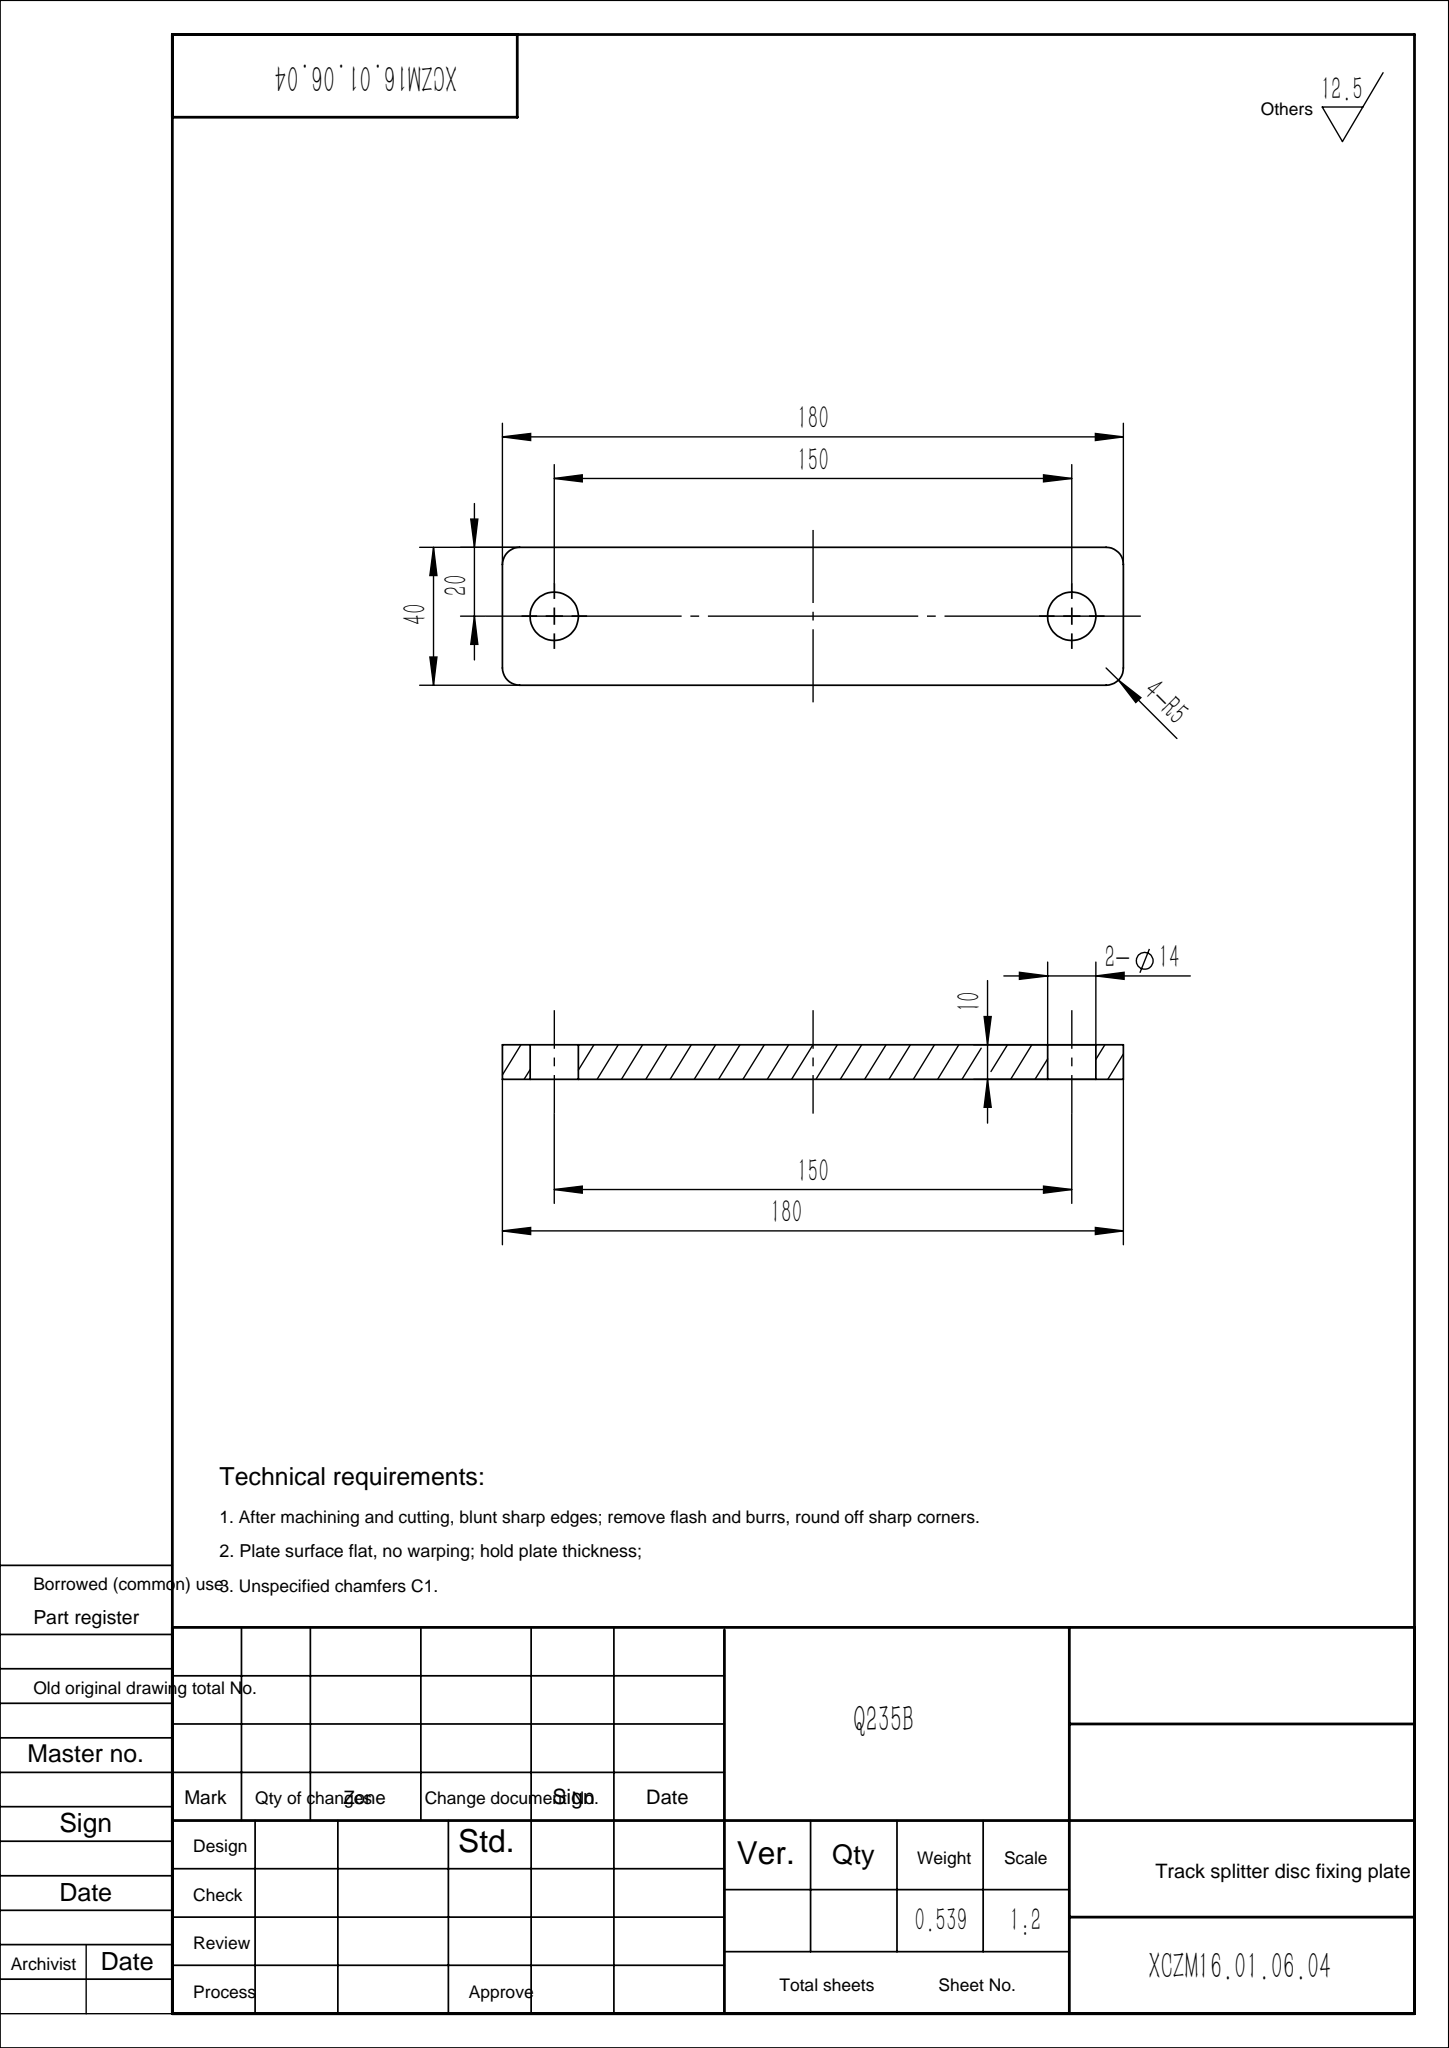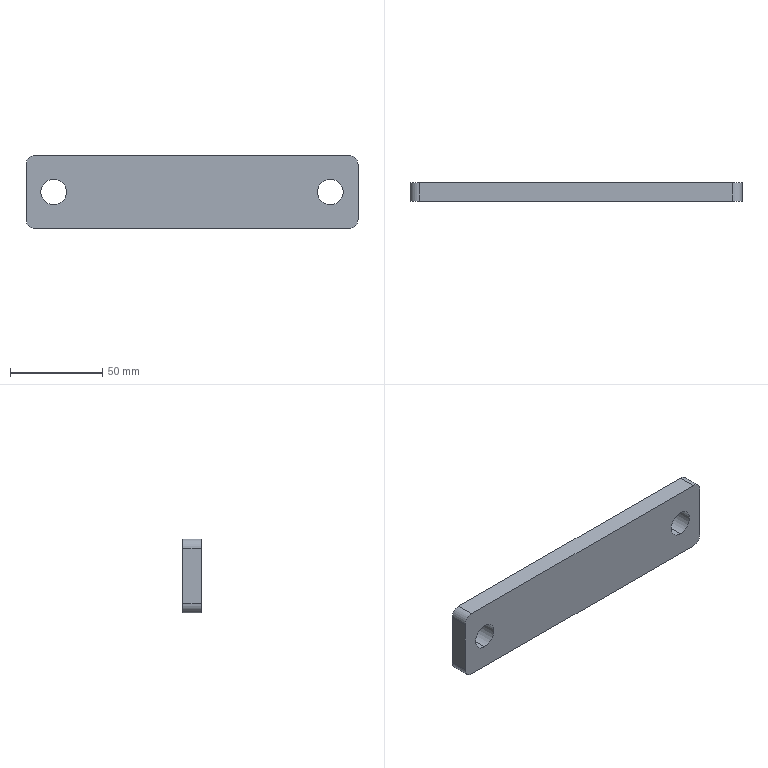Part | SolidWorks | features Extrusion 1 | 1 solid | 14 faces | box 180 x 10 x 40 mm | volume 68707 mm3 | cylinder 8 | plane 6 | commonest cylinder face diameters 10 x4 14 x4
STEP:
#1=CARTESIAN_POINT('',(75.,10.,-7.));
#2=VERTEX_POINT('',#1);
#3=CARTESIAN_POINT('',(75.,10.,7.));
#4=VERTEX_POINT('',#3);
#5=CARTESIAN_POINT('',(75.,10.,0.));
#6=DIRECTION('',(0.,1.,0.));
#7=DIRECTION('',(0.,0.,-1.));
#8=AXIS2_PLACEMENT_3D('',#5,#6,#7);
#9=CIRCLE('',#8,7.);
#10=EDGE_CURVE('',#2,#4,#9,.T.);
#11=ORIENTED_EDGE('',*,*,#10,.T.);
#12=CARTESIAN_POINT('',(75.,0.,7.));
#13=VERTEX_POINT('',#12);
#14=CARTESIAN_POINT('',(75.,10.,7.));
#15=DIRECTION('',(0.,-1.,0.));
#16=VECTOR('',#15,1000.);
#17=LINE('',#14,#16);
#18=EDGE_CURVE('',#4,#13,#17,.T.);
#19=ORIENTED_EDGE('',*,*,#18,.T.);
#20=CARTESIAN_POINT('',(75.,0.,-7.));
#21=VERTEX_POINT('',#20);
#22=CARTESIAN_POINT('',(75.,0.,0.));
#23=DIRECTION('',(0.,1.,0.));
#24=DIRECTION('',(0.,0.,-1.));
#25=AXIS2_PLACEMENT_3D('',#22,#23,#24);
#26=CIRCLE('',#25,7.);
#27=EDGE_CURVE('',#21,#13,#26,.T.);
#28=ORIENTED_EDGE('',*,*,#27,.F.);
#29=CARTESIAN_POINT('',(75.,10.,-7.));
#30=DIRECTION('',(0.,-1.,0.));
#31=VECTOR('',#30,1000.);
#32=LINE('',#29,#31);
#33=EDGE_CURVE('',#2,#21,#32,.T.);
#34=ORIENTED_EDGE('',*,*,#33,.F.);
#35=EDGE_LOOP('',(#11,#19,#28,#34));
#36=FACE_OUTER_BOUND('',#35,.T.);
#37=CARTESIAN_POINT('',(75.,10.,0.));
#38=DIRECTION('',(0.,-1.,0.));
#39=DIRECTION('',(0.,0.,-1.));
#40=AXIS2_PLACEMENT_3D('',#37,#38,#39);
#41=CYLINDRICAL_SURFACE('',#40,7.);
#42=ADVANCED_FACE('',(#36),#41,.F.);
#43=CARTESIAN_POINT('',(-75.,10.,-7.));
#44=VERTEX_POINT('',#43);
#45=CARTESIAN_POINT('',(-75.,10.,7.));
#46=VERTEX_POINT('',#45);
#47=CARTESIAN_POINT('',(-75.,10.,0.));
#48=DIRECTION('',(0.,1.,0.));
#49=DIRECTION('',(0.,0.,1.));
#50=AXIS2_PLACEMENT_3D('',#47,#48,#49);
#51=CIRCLE('',#50,7.);
#52=EDGE_CURVE('',#44,#46,#51,.T.);
#53=ORIENTED_EDGE('',*,*,#52,.T.);
#54=CARTESIAN_POINT('',(-75.,0.,7.));
#55=VERTEX_POINT('',#54);
#56=CARTESIAN_POINT('',(-75.,10.,7.));
#57=DIRECTION('',(0.,-1.,0.));
#58=VECTOR('',#57,1000.);
#59=LINE('',#56,#58);
#60=EDGE_CURVE('',#46,#55,#59,.T.);
#61=ORIENTED_EDGE('',*,*,#60,.T.);
#62=CARTESIAN_POINT('',(-75.,0.,-7.));
#63=VERTEX_POINT('',#62);
#64=CARTESIAN_POINT('',(-75.,0.,0.));
#65=DIRECTION('',(0.,1.,0.));
#66=DIRECTION('',(0.,0.,1.));
#67=AXIS2_PLACEMENT_3D('',#64,#65,#66);
#68=CIRCLE('',#67,7.);
#69=EDGE_CURVE('',#63,#55,#68,.T.);
#70=ORIENTED_EDGE('',*,*,#69,.F.);
#71=CARTESIAN_POINT('',(-75.,10.,-7.));
#72=DIRECTION('',(0.,-1.,0.));
#73=VECTOR('',#72,1000.);
#74=LINE('',#71,#73);
#75=EDGE_CURVE('',#44,#63,#74,.T.);
#76=ORIENTED_EDGE('',*,*,#75,.F.);
#77=EDGE_LOOP('',(#53,#61,#70,#76));
#78=FACE_OUTER_BOUND('',#77,.T.);
#79=CARTESIAN_POINT('',(-75.,10.,0.));
#80=DIRECTION('',(0.,-1.,0.));
#81=DIRECTION('',(0.,0.,-1.));
#82=AXIS2_PLACEMENT_3D('',#79,#80,#81);
#83=CYLINDRICAL_SURFACE('',#82,7.);
#84=ADVANCED_FACE('',(#78),#83,.F.);
#85=CARTESIAN_POINT('',(-90.,10.,15.));
#86=VERTEX_POINT('',#85);
#87=CARTESIAN_POINT('',(-85.,10.,20.));
#88=VERTEX_POINT('',#87);
#89=CARTESIAN_POINT('',(-85.,10.,15.));
#90=DIRECTION('',(0.,1.,0.));
#91=DIRECTION('',(0.,0.,-1.));
#92=AXIS2_PLACEMENT_3D('',#89,#90,#91);
#93=CIRCLE('',#92,5.);
#94=EDGE_CURVE('',#86,#88,#93,.T.);
#95=ORIENTED_EDGE('',*,*,#94,.T.);
#96=CARTESIAN_POINT('',(85.,10.,20.));
#97=VERTEX_POINT('',#96);
#98=CARTESIAN_POINT('',(85.,10.,20.));
#99=DIRECTION('',(1.,0.,0.));
#100=VECTOR('',#99,1000.);
#101=LINE('',#98,#100);
#102=EDGE_CURVE('',#88,#97,#101,.T.);
#103=ORIENTED_EDGE('',*,*,#102,.T.);
#104=CARTESIAN_POINT('',(90.,10.,15.));
#105=VERTEX_POINT('',#104);
#106=CARTESIAN_POINT('',(85.,10.,15.));
#107=DIRECTION('',(0.,1.,0.));
#108=DIRECTION('',(0.,0.,1.));
#109=AXIS2_PLACEMENT_3D('',#106,#107,#108);
#110=CIRCLE('',#109,5.);
#111=EDGE_CURVE('',#97,#105,#110,.T.);
#112=ORIENTED_EDGE('',*,*,#111,.T.);
#113=CARTESIAN_POINT('',(90.,10.,-15.));
#114=VERTEX_POINT('',#113);
#115=CARTESIAN_POINT('',(90.,10.,15.));
#116=DIRECTION('',(0.,0.,-1.));
#117=VECTOR('',#116,1000.);
#118=LINE('',#115,#117);
#119=EDGE_CURVE('',#105,#114,#118,.T.);
#120=ORIENTED_EDGE('',*,*,#119,.T.);
#121=CARTESIAN_POINT('',(85.,10.,-20.));
#122=VERTEX_POINT('',#121);
#123=CARTESIAN_POINT('',(85.,10.,-15.));
#124=DIRECTION('',(0.,1.,0.));
#125=DIRECTION('',(0.,0.,1.));
#126=AXIS2_PLACEMENT_3D('',#123,#124,#125);
#127=CIRCLE('',#126,5.);
#128=EDGE_CURVE('',#114,#122,#127,.T.);
#129=ORIENTED_EDGE('',*,*,#128,.T.);
#130=CARTESIAN_POINT('',(-85.,10.,-20.));
#131=VERTEX_POINT('',#130);
#132=CARTESIAN_POINT('',(85.,10.,-20.));
#133=DIRECTION('',(-1.,0.,0.));
#134=VECTOR('',#133,1000.);
#135=LINE('',#132,#134);
#136=EDGE_CURVE('',#122,#131,#135,.T.);
#137=ORIENTED_EDGE('',*,*,#136,.T.);
#138=CARTESIAN_POINT('',(-90.,10.,-15.));
#139=VERTEX_POINT('',#138);
#140=CARTESIAN_POINT('',(-85.,10.,-15.));
#141=DIRECTION('',(0.,1.,0.));
#142=DIRECTION('',(0.,0.,1.));
#143=AXIS2_PLACEMENT_3D('',#140,#141,#142);
#144=CIRCLE('',#143,5.);
#145=EDGE_CURVE('',#131,#139,#144,.T.);
#146=ORIENTED_EDGE('',*,*,#145,.T.);
#147=CARTESIAN_POINT('',(-90.,10.,15.));
#148=DIRECTION('',(0.,0.,1.));
#149=VECTOR('',#148,1000.);
#150=LINE('',#147,#149);
#151=EDGE_CURVE('',#139,#86,#150,.T.);
#152=ORIENTED_EDGE('',*,*,#151,.T.);
#153=EDGE_LOOP('',(#95,#103,#112,#120,#129,#137,#146,#152));
#154=FACE_OUTER_BOUND('',#153,.T.);
#155=ORIENTED_EDGE('',*,*,#52,.F.);
#156=CARTESIAN_POINT('',(-75.,10.,0.));
#157=DIRECTION('',(0.,1.,0.));
#158=DIRECTION('',(0.,0.,1.));
#159=AXIS2_PLACEMENT_3D('',#156,#157,#158);
#160=CIRCLE('',#159,7.);
#161=EDGE_CURVE('',#46,#44,#160,.T.);
#162=ORIENTED_EDGE('',*,*,#161,.F.);
#163=EDGE_LOOP('',(#155,#162));
#164=FACE_BOUND('',#163,.T.);
#165=ORIENTED_EDGE('',*,*,#10,.F.);
#166=CARTESIAN_POINT('',(75.,10.,0.));
#167=DIRECTION('',(0.,1.,0.));
#168=DIRECTION('',(0.,0.,-1.));
#169=AXIS2_PLACEMENT_3D('',#166,#167,#168);
#170=CIRCLE('',#169,7.);
#171=EDGE_CURVE('',#4,#2,#170,.T.);
#172=ORIENTED_EDGE('',*,*,#171,.F.);
#173=EDGE_LOOP('',(#165,#172));
#174=FACE_BOUND('',#173,.T.);
#175=CARTESIAN_POINT('',(-85.,10.,15.));
#176=DIRECTION('',(0.,-1.,0.));
#177=DIRECTION('',(0.,0.,-1.));
#178=AXIS2_PLACEMENT_3D('',#175,#176,#177);
#179=PLANE('',#178);
#180=ADVANCED_FACE('',(#154,#164,#174),#179,.F.);
#181=ORIENTED_EDGE('',*,*,#69,.T.);
#182=CARTESIAN_POINT('',(-75.,0.,0.));
#183=DIRECTION('',(0.,1.,0.));
#184=DIRECTION('',(0.,0.,1.));
#185=AXIS2_PLACEMENT_3D('',#182,#183,#184);
#186=CIRCLE('',#185,7.);
#187=EDGE_CURVE('',#55,#63,#186,.T.);
#188=ORIENTED_EDGE('',*,*,#187,.T.);
#189=EDGE_LOOP('',(#181,#188));
#190=FACE_BOUND('',#189,.T.);
#191=CARTESIAN_POINT('',(-90.,0.,15.));
#192=VERTEX_POINT('',#191);
#193=CARTESIAN_POINT('',(-85.,0.,20.));
#194=VERTEX_POINT('',#193);
#195=CARTESIAN_POINT('',(-85.,0.,15.));
#196=DIRECTION('',(0.,1.,0.));
#197=DIRECTION('',(0.,0.,-1.));
#198=AXIS2_PLACEMENT_3D('',#195,#196,#197);
#199=CIRCLE('',#198,5.);
#200=EDGE_CURVE('',#192,#194,#199,.T.);
#201=ORIENTED_EDGE('',*,*,#200,.F.);
#202=CARTESIAN_POINT('',(-90.,0.,-15.));
#203=VERTEX_POINT('',#202);
#204=CARTESIAN_POINT('',(-90.,0.,15.));
#205=DIRECTION('',(0.,0.,1.));
#206=VECTOR('',#205,1000.);
#207=LINE('',#204,#206);
#208=EDGE_CURVE('',#203,#192,#207,.T.);
#209=ORIENTED_EDGE('',*,*,#208,.F.);
#210=CARTESIAN_POINT('',(-85.,0.,-20.));
#211=VERTEX_POINT('',#210);
#212=CARTESIAN_POINT('',(-85.,0.,-15.));
#213=DIRECTION('',(0.,1.,0.));
#214=DIRECTION('',(0.,0.,1.));
#215=AXIS2_PLACEMENT_3D('',#212,#213,#214);
#216=CIRCLE('',#215,5.);
#217=EDGE_CURVE('',#211,#203,#216,.T.);
#218=ORIENTED_EDGE('',*,*,#217,.F.);
#219=CARTESIAN_POINT('',(85.,0.,-20.));
#220=VERTEX_POINT('',#219);
#221=CARTESIAN_POINT('',(85.,0.,-20.));
#222=DIRECTION('',(-1.,0.,0.));
#223=VECTOR('',#222,1000.);
#224=LINE('',#221,#223);
#225=EDGE_CURVE('',#220,#211,#224,.T.);
#226=ORIENTED_EDGE('',*,*,#225,.F.);
#227=CARTESIAN_POINT('',(90.,0.,-15.));
#228=VERTEX_POINT('',#227);
#229=CARTESIAN_POINT('',(85.,0.,-15.));
#230=DIRECTION('',(0.,1.,0.));
#231=DIRECTION('',(0.,0.,1.));
#232=AXIS2_PLACEMENT_3D('',#229,#230,#231);
#233=CIRCLE('',#232,5.);
#234=EDGE_CURVE('',#228,#220,#233,.T.);
#235=ORIENTED_EDGE('',*,*,#234,.F.);
#236=CARTESIAN_POINT('',(90.,0.,15.));
#237=VERTEX_POINT('',#236);
#238=CARTESIAN_POINT('',(90.,0.,15.));
#239=DIRECTION('',(0.,0.,-1.));
#240=VECTOR('',#239,1000.);
#241=LINE('',#238,#240);
#242=EDGE_CURVE('',#237,#228,#241,.T.);
#243=ORIENTED_EDGE('',*,*,#242,.F.);
#244=CARTESIAN_POINT('',(85.,0.,20.));
#245=VERTEX_POINT('',#244);
#246=CARTESIAN_POINT('',(85.,0.,15.));
#247=DIRECTION('',(0.,1.,0.));
#248=DIRECTION('',(0.,0.,1.));
#249=AXIS2_PLACEMENT_3D('',#246,#247,#248);
#250=CIRCLE('',#249,5.);
#251=EDGE_CURVE('',#245,#237,#250,.T.);
#252=ORIENTED_EDGE('',*,*,#251,.F.);
#253=CARTESIAN_POINT('',(85.,0.,20.));
#254=DIRECTION('',(1.,0.,0.));
#255=VECTOR('',#254,1000.);
#256=LINE('',#253,#255);
#257=EDGE_CURVE('',#194,#245,#256,.T.);
#258=ORIENTED_EDGE('',*,*,#257,.F.);
#259=EDGE_LOOP('',(#201,#209,#218,#226,#235,#243,#252,#258));
#260=FACE_OUTER_BOUND('',#259,.T.);
#261=ORIENTED_EDGE('',*,*,#27,.T.);
#262=CARTESIAN_POINT('',(75.,0.,0.));
#263=DIRECTION('',(0.,1.,0.));
#264=DIRECTION('',(0.,0.,-1.));
#265=AXIS2_PLACEMENT_3D('',#262,#263,#264);
#266=CIRCLE('',#265,7.);
#267=EDGE_CURVE('',#13,#21,#266,.T.);
#268=ORIENTED_EDGE('',*,*,#267,.T.);
#269=EDGE_LOOP('',(#261,#268));
#270=FACE_BOUND('',#269,.T.);
#271=CARTESIAN_POINT('',(-85.,0.,15.));
#272=DIRECTION('',(0.,-1.,0.));
#273=DIRECTION('',(0.,0.,-1.));
#274=AXIS2_PLACEMENT_3D('',#271,#272,#273);
#275=PLANE('',#274);
#276=ADVANCED_FACE('',(#190,#260,#270),#275,.T.);
#277=ORIENTED_EDGE('',*,*,#200,.T.);
#278=CARTESIAN_POINT('',(-85.,10.,20.));
#279=DIRECTION('',(0.,-1.,0.));
#280=VECTOR('',#279,1000.);
#281=LINE('',#278,#280);
#282=EDGE_CURVE('',#88,#194,#281,.T.);
#283=ORIENTED_EDGE('',*,*,#282,.F.);
#284=ORIENTED_EDGE('',*,*,#94,.F.);
#285=CARTESIAN_POINT('',(-90.,10.,15.));
#286=DIRECTION('',(0.,-1.,0.));
#287=VECTOR('',#286,1000.);
#288=LINE('',#285,#287);
#289=EDGE_CURVE('',#86,#192,#288,.T.);
#290=ORIENTED_EDGE('',*,*,#289,.T.);
#291=EDGE_LOOP('',(#277,#283,#284,#290));
#292=FACE_OUTER_BOUND('',#291,.T.);
#293=CARTESIAN_POINT('',(-85.,10.,15.));
#294=DIRECTION('',(0.,-1.,0.));
#295=DIRECTION('',(0.,0.,-1.));
#296=AXIS2_PLACEMENT_3D('',#293,#294,#295);
#297=CYLINDRICAL_SURFACE('',#296,5.);
#298=ADVANCED_FACE('',(#292),#297,.T.);
#299=ORIENTED_EDGE('',*,*,#257,.T.);
#300=CARTESIAN_POINT('',(85.,10.,20.));
#301=DIRECTION('',(0.,-1.,0.));
#302=VECTOR('',#301,1000.);
#303=LINE('',#300,#302);
#304=EDGE_CURVE('',#97,#245,#303,.T.);
#305=ORIENTED_EDGE('',*,*,#304,.F.);
#306=ORIENTED_EDGE('',*,*,#102,.F.);
#307=ORIENTED_EDGE('',*,*,#282,.T.);
#308=EDGE_LOOP('',(#299,#305,#306,#307));
#309=FACE_OUTER_BOUND('',#308,.T.);
#310=CARTESIAN_POINT('',(85.,10.,20.));
#311=DIRECTION('',(0.,0.,-1.));
#312=DIRECTION('',(-1.,0.,0.));
#313=AXIS2_PLACEMENT_3D('',#310,#311,#312);
#314=PLANE('',#313);
#315=ADVANCED_FACE('',(#309),#314,.F.);
#316=ORIENTED_EDGE('',*,*,#251,.T.);
#317=CARTESIAN_POINT('',(90.,10.,15.));
#318=DIRECTION('',(0.,-1.,0.));
#319=VECTOR('',#318,1000.);
#320=LINE('',#317,#319);
#321=EDGE_CURVE('',#105,#237,#320,.T.);
#322=ORIENTED_EDGE('',*,*,#321,.F.);
#323=ORIENTED_EDGE('',*,*,#111,.F.);
#324=ORIENTED_EDGE('',*,*,#304,.T.);
#325=EDGE_LOOP('',(#316,#322,#323,#324));
#326=FACE_OUTER_BOUND('',#325,.T.);
#327=CARTESIAN_POINT('',(85.,10.,15.));
#328=DIRECTION('',(0.,-1.,0.));
#329=DIRECTION('',(0.,0.,-1.));
#330=AXIS2_PLACEMENT_3D('',#327,#328,#329);
#331=CYLINDRICAL_SURFACE('',#330,5.);
#332=ADVANCED_FACE('',(#326),#331,.T.);
#333=ORIENTED_EDGE('',*,*,#242,.T.);
#334=CARTESIAN_POINT('',(90.,10.,-15.));
#335=DIRECTION('',(0.,-1.,0.));
#336=VECTOR('',#335,1000.);
#337=LINE('',#334,#336);
#338=EDGE_CURVE('',#114,#228,#337,.T.);
#339=ORIENTED_EDGE('',*,*,#338,.F.);
#340=ORIENTED_EDGE('',*,*,#119,.F.);
#341=ORIENTED_EDGE('',*,*,#321,.T.);
#342=EDGE_LOOP('',(#333,#339,#340,#341));
#343=FACE_OUTER_BOUND('',#342,.T.);
#344=CARTESIAN_POINT('',(90.,10.,15.));
#345=DIRECTION('',(-1.,0.,0.));
#346=DIRECTION('',(0.,0.,1.));
#347=AXIS2_PLACEMENT_3D('',#344,#345,#346);
#348=PLANE('',#347);
#349=ADVANCED_FACE('',(#343),#348,.F.);
#350=ORIENTED_EDGE('',*,*,#234,.T.);
#351=CARTESIAN_POINT('',(85.,10.,-20.));
#352=DIRECTION('',(0.,-1.,0.));
#353=VECTOR('',#352,1000.);
#354=LINE('',#351,#353);
#355=EDGE_CURVE('',#122,#220,#354,.T.);
#356=ORIENTED_EDGE('',*,*,#355,.F.);
#357=ORIENTED_EDGE('',*,*,#128,.F.);
#358=ORIENTED_EDGE('',*,*,#338,.T.);
#359=EDGE_LOOP('',(#350,#356,#357,#358));
#360=FACE_OUTER_BOUND('',#359,.T.);
#361=CARTESIAN_POINT('',(85.,10.,-15.));
#362=DIRECTION('',(0.,-1.,0.));
#363=DIRECTION('',(0.,0.,-1.));
#364=AXIS2_PLACEMENT_3D('',#361,#362,#363);
#365=CYLINDRICAL_SURFACE('',#364,5.);
#366=ADVANCED_FACE('',(#360),#365,.T.);
#367=ORIENTED_EDGE('',*,*,#225,.T.);
#368=CARTESIAN_POINT('',(-85.,10.,-20.));
#369=DIRECTION('',(0.,-1.,0.));
#370=VECTOR('',#369,1000.);
#371=LINE('',#368,#370);
#372=EDGE_CURVE('',#131,#211,#371,.T.);
#373=ORIENTED_EDGE('',*,*,#372,.F.);
#374=ORIENTED_EDGE('',*,*,#136,.F.);
#375=ORIENTED_EDGE('',*,*,#355,.T.);
#376=EDGE_LOOP('',(#367,#373,#374,#375));
#377=FACE_OUTER_BOUND('',#376,.T.);
#378=CARTESIAN_POINT('',(85.,10.,-20.));
#379=DIRECTION('',(0.,0.,1.));
#380=DIRECTION('',(1.,0.,0.));
#381=AXIS2_PLACEMENT_3D('',#378,#379,#380);
#382=PLANE('',#381);
#383=ADVANCED_FACE('',(#377),#382,.F.);
#384=ORIENTED_EDGE('',*,*,#217,.T.);
#385=CARTESIAN_POINT('',(-90.,10.,-15.));
#386=DIRECTION('',(0.,-1.,0.));
#387=VECTOR('',#386,1000.);
#388=LINE('',#385,#387);
#389=EDGE_CURVE('',#139,#203,#388,.T.);
#390=ORIENTED_EDGE('',*,*,#389,.F.);
#391=ORIENTED_EDGE('',*,*,#145,.F.);
#392=ORIENTED_EDGE('',*,*,#372,.T.);
#393=EDGE_LOOP('',(#384,#390,#391,#392));
#394=FACE_OUTER_BOUND('',#393,.T.);
#395=CARTESIAN_POINT('',(-85.,10.,-15.));
#396=DIRECTION('',(0.,-1.,0.));
#397=DIRECTION('',(0.,0.,-1.));
#398=AXIS2_PLACEMENT_3D('',#395,#396,#397);
#399=CYLINDRICAL_SURFACE('',#398,5.);
#400=ADVANCED_FACE('',(#394),#399,.T.);
#401=ORIENTED_EDGE('',*,*,#208,.T.);
#402=ORIENTED_EDGE('',*,*,#289,.F.);
#403=ORIENTED_EDGE('',*,*,#151,.F.);
#404=ORIENTED_EDGE('',*,*,#389,.T.);
#405=EDGE_LOOP('',(#401,#402,#403,#404));
#406=FACE_OUTER_BOUND('',#405,.T.);
#407=CARTESIAN_POINT('',(-90.,10.,15.));
#408=DIRECTION('',(1.,0.,0.));
#409=DIRECTION('',(0.,0.,-1.));
#410=AXIS2_PLACEMENT_3D('',#407,#408,#409);
#411=PLANE('',#410);
#412=ADVANCED_FACE('',(#406),#411,.F.);
#413=ORIENTED_EDGE('',*,*,#60,.F.);
#414=ORIENTED_EDGE('',*,*,#161,.T.);
#415=ORIENTED_EDGE('',*,*,#75,.T.);
#416=ORIENTED_EDGE('',*,*,#187,.F.);
#417=EDGE_LOOP('',(#413,#414,#415,#416));
#418=FACE_OUTER_BOUND('',#417,.T.);
#419=CARTESIAN_POINT('',(-75.,10.,0.));
#420=DIRECTION('',(0.,-1.,0.));
#421=DIRECTION('',(0.,0.,-1.));
#422=AXIS2_PLACEMENT_3D('',#419,#420,#421);
#423=CYLINDRICAL_SURFACE('',#422,7.);
#424=ADVANCED_FACE('',(#418),#423,.F.);
#425=ORIENTED_EDGE('',*,*,#18,.F.);
#426=ORIENTED_EDGE('',*,*,#171,.T.);
#427=ORIENTED_EDGE('',*,*,#33,.T.);
#428=ORIENTED_EDGE('',*,*,#267,.F.);
#429=EDGE_LOOP('',(#425,#426,#427,#428));
#430=FACE_OUTER_BOUND('',#429,.T.);
#431=CARTESIAN_POINT('',(75.,10.,0.));
#432=DIRECTION('',(0.,-1.,0.));
#433=DIRECTION('',(0.,0.,-1.));
#434=AXIS2_PLACEMENT_3D('',#431,#432,#433);
#435=CYLINDRICAL_SURFACE('',#434,7.);
#436=ADVANCED_FACE('',(#430),#435,.F.);
#437=CLOSED_SHELL('',(#42,#84,#180,#276,#298,#315,#332,#349,#366,#383,#400,#412,#424,#436));
#438=MANIFOLD_SOLID_BREP('',#437);
#439=CARTESIAN_POINT('',(0.,0.,0.));
#440=DIRECTION('',(0.,0.,1.));
#441=DIRECTION('',(1.,0.,0.));
#442=AXIS2_PLACEMENT_3D('',#439,#440,#441);
#443=(LENGTH_UNIT()NAMED_UNIT(*)SI_UNIT(.MILLI.,.METRE.));
#444=UNCERTAINTY_MEASURE_WITH_UNIT(LENGTH_MEASURE(0.00001),#443,'','');
#445=(NAMED_UNIT(*)PLANE_ANGLE_UNIT()SI_UNIT($,.RADIAN.));
#446=(NAMED_UNIT(*)SI_UNIT($,.STERADIAN.)SOLID_ANGLE_UNIT());
#447=(GEOMETRIC_REPRESENTATION_CONTEXT(3)GLOBAL_UNCERTAINTY_ASSIGNED_CONTEXT((#444))GLOBAL_UNIT_ASSIGNED_CONTEXT((#443,#445,#446))REPRESENTATION_CONTEXT('',''));
#448=ADVANCED_BREP_SHAPE_REPRESENTATION('',(#438,#442),#447);